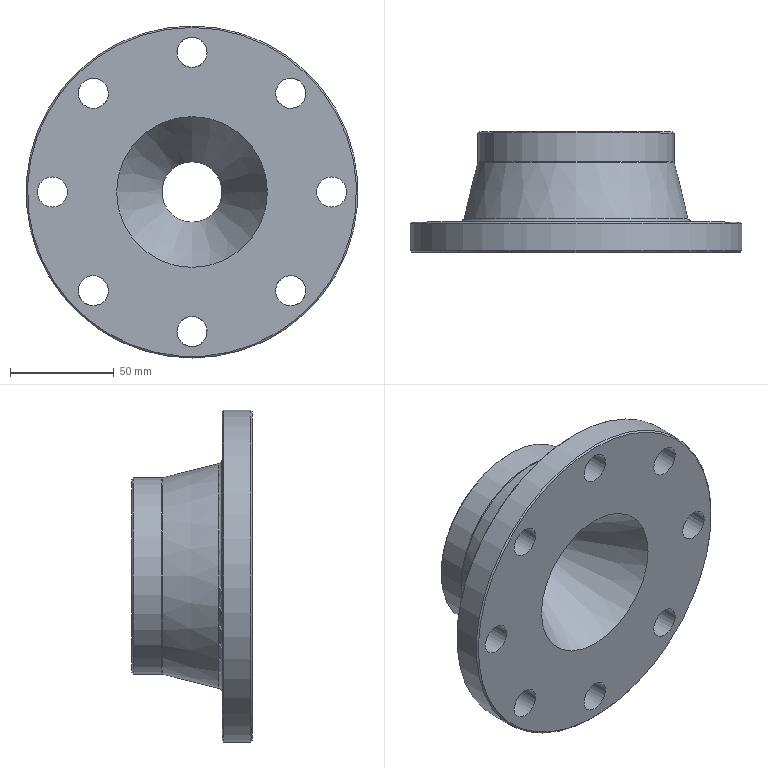Part | NX | features INSTANCE 8, ABSOLUTE_DATUM_PLANE 3, CHAMFER 2, DATUM_CSYS 2, SKETCH 2, ABSOLUTE_DATUM_AXIS 1, BLEND 1, CIRCULAR_ISET 1, HOLE PACKAGE 1, SCALE 1, SIMPLE HOLE 1, SWP104 1, TRANSFORM_ISET 1 | 1 solid | 21 faces | box 160 x 58.182 x 160 mm | volume 514948 mm3 | cylinder 11 | cone 5 | plane 3 | torus 2 | commonest cylinder face diameters 14.545 x8 29.091 x1 94.545 x1 160 x1
STEP:
#1=CARTESIAN_POINT('',(0.,17.422,79.273));
#2=VERTEX_POINT('',#1);
#3=CARTESIAN_POINT('',(0.,17.422,0.));
#4=DIRECTION('',(0.,1.,0.));
#5=DIRECTION('',(0.,0.,1.));
#6=AXIS2_PLACEMENT_3D('',#3,#4,#5);
#7=CIRCLE('',#6,79.273);
#8=EDGE_CURVE('',#2,#2,#7,.F.);
#9=ORIENTED_EDGE('',*,*,#8,.T.);
#10=EDGE_LOOP('',(#9));
#11=FACE_BOUND('',#10,.T.);
#12=CARTESIAN_POINT('',(47.569,17.422,54.842));
#13=VERTEX_POINT('',#12);
#14=CARTESIAN_POINT('',(47.569,17.422,47.569));
#15=DIRECTION('',(0.,1.,0.));
#16=DIRECTION('',(0.,0.,1.));
#17=AXIS2_PLACEMENT_3D('',#14,#15,#16);
#18=CIRCLE('',#17,7.273);
#19=EDGE_CURVE('',#13,#13,#18,.T.);
#20=ORIENTED_EDGE('',*,*,#19,.T.);
#21=EDGE_LOOP('',(#20));
#22=FACE_BOUND('',#21,.T.);
#23=CARTESIAN_POINT('',(0.,17.422,74.545));
#24=VERTEX_POINT('',#23);
#25=CARTESIAN_POINT('',(0.,17.422,67.273));
#26=DIRECTION('',(0.,1.,0.));
#27=DIRECTION('',(0.,0.,1.));
#28=AXIS2_PLACEMENT_3D('',#25,#26,#27);
#29=CIRCLE('',#28,7.273);
#30=EDGE_CURVE('',#24,#24,#29,.T.);
#31=ORIENTED_EDGE('',*,*,#30,.T.);
#32=EDGE_LOOP('',(#31));
#33=FACE_BOUND('',#32,.T.);
#34=CARTESIAN_POINT('',(-47.569,17.422,54.842));
#35=VERTEX_POINT('',#34);
#36=CARTESIAN_POINT('',(-47.569,17.422,47.569));
#37=DIRECTION('',(0.,1.,0.));
#38=DIRECTION('',(0.,0.,1.));
#39=AXIS2_PLACEMENT_3D('',#36,#37,#38);
#40=CIRCLE('',#39,7.273);
#41=EDGE_CURVE('',#35,#35,#40,.T.);
#42=ORIENTED_EDGE('',*,*,#41,.T.);
#43=EDGE_LOOP('',(#42));
#44=FACE_BOUND('',#43,.T.);
#45=CARTESIAN_POINT('',(-67.273,17.422,7.273));
#46=VERTEX_POINT('',#45);
#47=CARTESIAN_POINT('',(-67.273,17.422,0.));
#48=DIRECTION('',(0.,1.,0.));
#49=DIRECTION('',(0.,0.,1.));
#50=AXIS2_PLACEMENT_3D('',#47,#48,#49);
#51=CIRCLE('',#50,7.273);
#52=EDGE_CURVE('',#46,#46,#51,.T.);
#53=ORIENTED_EDGE('',*,*,#52,.T.);
#54=EDGE_LOOP('',(#53));
#55=FACE_BOUND('',#54,.T.);
#56=CARTESIAN_POINT('',(-47.569,17.422,-40.296));
#57=VERTEX_POINT('',#56);
#58=CARTESIAN_POINT('',(-47.569,17.422,-47.569));
#59=DIRECTION('',(0.,1.,0.));
#60=DIRECTION('',(0.,0.,1.));
#61=AXIS2_PLACEMENT_3D('',#58,#59,#60);
#62=CIRCLE('',#61,7.273);
#63=EDGE_CURVE('',#57,#57,#62,.T.);
#64=ORIENTED_EDGE('',*,*,#63,.T.);
#65=EDGE_LOOP('',(#64));
#66=FACE_BOUND('',#65,.T.);
#67=CARTESIAN_POINT('',(0.,17.422,-60.));
#68=VERTEX_POINT('',#67);
#69=CARTESIAN_POINT('',(0.,17.422,-67.273));
#70=DIRECTION('',(0.,1.,0.));
#71=DIRECTION('',(0.,0.,1.));
#72=AXIS2_PLACEMENT_3D('',#69,#70,#71);
#73=CIRCLE('',#72,7.273);
#74=EDGE_CURVE('',#68,#68,#73,.T.);
#75=ORIENTED_EDGE('',*,*,#74,.T.);
#76=EDGE_LOOP('',(#75));
#77=FACE_BOUND('',#76,.T.);
#78=CARTESIAN_POINT('',(47.569,17.422,-40.296));
#79=VERTEX_POINT('',#78);
#80=CARTESIAN_POINT('',(47.569,17.422,-47.569));
#81=DIRECTION('',(0.,1.,0.));
#82=DIRECTION('',(0.,0.,1.));
#83=AXIS2_PLACEMENT_3D('',#80,#81,#82);
#84=CIRCLE('',#83,7.273);
#85=EDGE_CURVE('',#79,#79,#84,.T.);
#86=ORIENTED_EDGE('',*,*,#85,.T.);
#87=EDGE_LOOP('',(#86));
#88=FACE_BOUND('',#87,.T.);
#89=CARTESIAN_POINT('',(67.273,17.422,7.273));
#90=VERTEX_POINT('',#89);
#91=CARTESIAN_POINT('',(67.273,17.422,0.));
#92=DIRECTION('',(0.,1.,0.));
#93=DIRECTION('',(0.,0.,1.));
#94=AXIS2_PLACEMENT_3D('',#91,#92,#93);
#95=CIRCLE('',#94,7.273);
#96=EDGE_CURVE('',#90,#90,#95,.T.);
#97=ORIENTED_EDGE('',*,*,#96,.T.);
#98=EDGE_LOOP('',(#97));
#99=FACE_BOUND('',#98,.T.);
#100=CARTESIAN_POINT('',(0.,17.422,-36.364));
#101=VERTEX_POINT('',#100);
#102=CARTESIAN_POINT('',(0.,17.422,0.));
#103=DIRECTION('',(0.,-1.,0.));
#104=DIRECTION('',(0.,0.,-1.));
#105=AXIS2_PLACEMENT_3D('',#102,#103,#104);
#106=CIRCLE('',#105,36.364);
#107=EDGE_CURVE('',#101,#101,#106,.T.);
#108=ORIENTED_EDGE('',*,*,#107,.F.);
#109=EDGE_LOOP('',(#108));
#110=FACE_BOUND('',#109,.T.);
#111=CARTESIAN_POINT('',(80.,17.422,0.));
#112=DIRECTION('',(0.,1.,0.));
#113=DIRECTION('',(0.,0.,1.));
#114=AXIS2_PLACEMENT_3D('',#111,#112,#113);
#115=PLANE('',#114);
#116=ADVANCED_FACE('',(#11,#22,#33,#44,#55,#66,#77,#88,#99,#110),#115,.F.);
#117=CARTESIAN_POINT('',(0.,56.695,-14.545));
#118=VERTEX_POINT('',#117);
#119=CARTESIAN_POINT('',(0.,56.695,0.));
#120=DIRECTION('',(0.,-1.,0.));
#121=DIRECTION('',(0.,0.,-1.));
#122=AXIS2_PLACEMENT_3D('',#119,#120,#121);
#123=CIRCLE('',#122,14.545);
#124=EDGE_CURVE('',#118,#118,#123,.T.);
#125=ORIENTED_EDGE('',*,*,#124,.F.);
#126=EDGE_LOOP('',(#125));
#127=FACE_BOUND('',#126,.T.);
#128=ORIENTED_EDGE('',*,*,#107,.T.);
#129=EDGE_LOOP('',(#128));
#130=FACE_BOUND('',#129,.T.);
#131=CARTESIAN_POINT('',(0.,17.422,0.));
#132=DIRECTION('',(0.,-1.,0.));
#133=DIRECTION('',(0.,0.,-1.));
#134=AXIS2_PLACEMENT_3D('',#131,#132,#133);
#135=CONICAL_SURFACE('',#134,36.364,0.5071);
#136=ADVANCED_FACE('',(#127,#130),#135,.F.);
#137=CARTESIAN_POINT('',(0.,75.604,-14.545));
#138=VERTEX_POINT('',#137);
#139=CARTESIAN_POINT('',(0.,75.604,0.));
#140=DIRECTION('',(0.,-1.,0.));
#141=DIRECTION('',(0.,0.,-1.));
#142=AXIS2_PLACEMENT_3D('',#139,#140,#141);
#143=CIRCLE('',#142,14.545);
#144=EDGE_CURVE('',#138,#138,#143,.T.);
#145=ORIENTED_EDGE('',*,*,#144,.F.);
#146=EDGE_LOOP('',(#145));
#147=FACE_BOUND('',#146,.T.);
#148=ORIENTED_EDGE('',*,*,#124,.T.);
#149=EDGE_LOOP('',(#148));
#150=FACE_BOUND('',#149,.T.);
#151=CARTESIAN_POINT('',(0.,0.,0.));
#152=DIRECTION('',(0.,-1.,0.));
#153=DIRECTION('',(0.,0.,-1.));
#154=AXIS2_PLACEMENT_3D('',#151,#152,#153);
#155=CYLINDRICAL_SURFACE('',#154,14.545);
#156=ADVANCED_FACE('',(#147,#150),#155,.F.);
#157=CARTESIAN_POINT('',(0.,75.604,-46.545));
#158=VERTEX_POINT('',#157);
#159=CARTESIAN_POINT('',(0.,75.604,0.));
#160=DIRECTION('',(0.,-1.,0.));
#161=DIRECTION('',(0.,0.,-1.));
#162=AXIS2_PLACEMENT_3D('',#159,#160,#161);
#163=CIRCLE('',#162,46.545);
#164=EDGE_CURVE('',#158,#158,#163,.F.);
#165=ORIENTED_EDGE('',*,*,#164,.T.);
#166=EDGE_LOOP('',(#165));
#167=FACE_BOUND('',#166,.T.);
#168=ORIENTED_EDGE('',*,*,#144,.T.);
#169=EDGE_LOOP('',(#168));
#170=FACE_BOUND('',#169,.T.);
#171=CARTESIAN_POINT('',(14.545,75.604,0.));
#172=DIRECTION('',(0.,-1.,0.));
#173=DIRECTION('',(0.,0.,-1.));
#174=AXIS2_PLACEMENT_3D('',#171,#172,#173);
#175=PLANE('',#174);
#176=ADVANCED_FACE('',(#167,#170),#175,.F.);
#177=CARTESIAN_POINT('',(0.,61.327,-47.273));
#178=VERTEX_POINT('',#177);
#179=CARTESIAN_POINT('',(0.,61.327,0.));
#180=DIRECTION('',(0.,-1.,0.));
#181=DIRECTION('',(0.,0.,-1.));
#182=AXIS2_PLACEMENT_3D('',#179,#180,#181);
#183=CIRCLE('',#182,47.273);
#184=EDGE_CURVE('',#178,#178,#183,.F.);
#185=ORIENTED_EDGE('',*,*,#184,.T.);
#186=EDGE_LOOP('',(#185));
#187=FACE_BOUND('',#186,.T.);
#188=CARTESIAN_POINT('',(0.,74.877,-47.273));
#189=VERTEX_POINT('',#188);
#190=CARTESIAN_POINT('',(0.,74.877,0.));
#191=DIRECTION('',(0.,-1.,0.));
#192=DIRECTION('',(0.,0.,-1.));
#193=AXIS2_PLACEMENT_3D('',#190,#191,#192);
#194=CIRCLE('',#193,47.273);
#195=EDGE_CURVE('',#189,#189,#194,.T.);
#196=ORIENTED_EDGE('',*,*,#195,.T.);
#197=EDGE_LOOP('',(#196));
#198=FACE_BOUND('',#197,.T.);
#199=CARTESIAN_POINT('',(0.,0.,0.));
#200=DIRECTION('',(0.,-1.,0.));
#201=DIRECTION('',(0.,0.,-1.));
#202=AXIS2_PLACEMENT_3D('',#199,#200,#201);
#203=CYLINDRICAL_SURFACE('',#202,47.273);
#204=ADVANCED_FACE('',(#187,#198),#203,.T.);
#205=CARTESIAN_POINT('',(0.,33.62,-54.132));
#206=VERTEX_POINT('',#205);
#207=CARTESIAN_POINT('',(0.,33.62,0.));
#208=DIRECTION('',(0.,-1.,0.));
#209=DIRECTION('',(0.,0.,-1.));
#210=AXIS2_PLACEMENT_3D('',#207,#208,#209);
#211=CIRCLE('',#210,54.132);
#212=EDGE_CURVE('',#206,#206,#211,.F.);
#213=ORIENTED_EDGE('',*,*,#212,.T.);
#214=EDGE_LOOP('',(#213));
#215=FACE_BOUND('',#214,.T.);
#216=CARTESIAN_POINT('',(0.,60.798,-47.338));
#217=VERTEX_POINT('',#216);
#218=CARTESIAN_POINT('',(0.,60.798,0.));
#219=DIRECTION('',(0.,-1.,0.));
#220=DIRECTION('',(0.,0.,-1.));
#221=AXIS2_PLACEMENT_3D('',#218,#219,#220);
#222=CIRCLE('',#221,47.338);
#223=EDGE_CURVE('',#217,#217,#222,.T.);
#224=ORIENTED_EDGE('',*,*,#223,.T.);
#225=EDGE_LOOP('',(#224));
#226=FACE_BOUND('',#225,.T.);
#227=CARTESIAN_POINT('',(0.,61.059,0.));
#228=DIRECTION('',(0.,-1.,0.));
#229=DIRECTION('',(0.,0.,-1.));
#230=AXIS2_PLACEMENT_3D('',#227,#228,#229);
#231=CONICAL_SURFACE('',#230,47.273,0.245);
#232=ADVANCED_FACE('',(#215,#226),#231,.T.);
#233=CARTESIAN_POINT('',(52.712,31.968,42.426));
#234=VERTEX_POINT('',#233);
#235=CARTESIAN_POINT('',(47.569,31.968,47.569));
#236=DIRECTION('',(0.,-1.,0.));
#237=DIRECTION('',(0.7071,0.,-0.7071));
#238=AXIS2_PLACEMENT_3D('',#235,#236,#237);
#239=CIRCLE('',#238,7.273);
#240=EDGE_CURVE('',#234,#234,#239,.T.);
#241=ORIENTED_EDGE('',*,*,#240,.T.);
#242=EDGE_LOOP('',(#241));
#243=FACE_BOUND('',#242,.T.);
#244=CARTESIAN_POINT('',(7.273,31.968,67.273));
#245=VERTEX_POINT('',#244);
#246=CARTESIAN_POINT('',(0.,31.968,67.273));
#247=DIRECTION('',(0.,-1.,0.));
#248=DIRECTION('',(1.,0.,0.));
#249=AXIS2_PLACEMENT_3D('',#246,#247,#248);
#250=CIRCLE('',#249,7.273);
#251=EDGE_CURVE('',#245,#245,#250,.T.);
#252=ORIENTED_EDGE('',*,*,#251,.T.);
#253=EDGE_LOOP('',(#252));
#254=FACE_BOUND('',#253,.T.);
#255=CARTESIAN_POINT('',(-42.426,31.968,52.712));
#256=VERTEX_POINT('',#255);
#257=CARTESIAN_POINT('',(-47.569,31.968,47.569));
#258=DIRECTION('',(0.,-1.,0.));
#259=DIRECTION('',(0.7071,0.,0.7071));
#260=AXIS2_PLACEMENT_3D('',#257,#258,#259);
#261=CIRCLE('',#260,7.273);
#262=EDGE_CURVE('',#256,#256,#261,.T.);
#263=ORIENTED_EDGE('',*,*,#262,.T.);
#264=EDGE_LOOP('',(#263));
#265=FACE_BOUND('',#264,.T.);
#266=CARTESIAN_POINT('',(-67.273,31.968,7.273));
#267=VERTEX_POINT('',#266);
#268=CARTESIAN_POINT('',(-67.273,31.968,0.));
#269=DIRECTION('',(0.,-1.,0.));
#270=DIRECTION('',(0.,0.,1.));
#271=AXIS2_PLACEMENT_3D('',#268,#269,#270);
#272=CIRCLE('',#271,7.273);
#273=EDGE_CURVE('',#267,#267,#272,.T.);
#274=ORIENTED_EDGE('',*,*,#273,.T.);
#275=EDGE_LOOP('',(#274));
#276=FACE_BOUND('',#275,.T.);
#277=CARTESIAN_POINT('',(-52.712,31.968,-42.426));
#278=VERTEX_POINT('',#277);
#279=CARTESIAN_POINT('',(-47.569,31.968,-47.569));
#280=DIRECTION('',(0.,-1.,0.));
#281=DIRECTION('',(-0.7071,0.,0.7071));
#282=AXIS2_PLACEMENT_3D('',#279,#280,#281);
#283=CIRCLE('',#282,7.273);
#284=EDGE_CURVE('',#278,#278,#283,.T.);
#285=ORIENTED_EDGE('',*,*,#284,.T.);
#286=EDGE_LOOP('',(#285));
#287=FACE_BOUND('',#286,.T.);
#288=CARTESIAN_POINT('',(-7.273,31.968,-67.273));
#289=VERTEX_POINT('',#288);
#290=CARTESIAN_POINT('',(0.,31.968,-67.273));
#291=DIRECTION('',(0.,-1.,0.));
#292=DIRECTION('',(-1.,0.,0.));
#293=AXIS2_PLACEMENT_3D('',#290,#291,#292);
#294=CIRCLE('',#293,7.273);
#295=EDGE_CURVE('',#289,#289,#294,.T.);
#296=ORIENTED_EDGE('',*,*,#295,.T.);
#297=EDGE_LOOP('',(#296));
#298=FACE_BOUND('',#297,.T.);
#299=CARTESIAN_POINT('',(42.426,31.968,-52.712));
#300=VERTEX_POINT('',#299);
#301=CARTESIAN_POINT('',(47.569,31.968,-47.569));
#302=DIRECTION('',(0.,-1.,0.));
#303=DIRECTION('',(-0.7071,0.,-0.7071));
#304=AXIS2_PLACEMENT_3D('',#301,#302,#303);
#305=CIRCLE('',#304,7.273);
#306=EDGE_CURVE('',#300,#300,#305,.T.);
#307=ORIENTED_EDGE('',*,*,#306,.T.);
#308=EDGE_LOOP('',(#307));
#309=FACE_BOUND('',#308,.T.);
#310=CARTESIAN_POINT('',(67.273,31.968,-7.273));
#311=VERTEX_POINT('',#310);
#312=CARTESIAN_POINT('',(67.273,31.968,0.));
#313=DIRECTION('',(0.,-1.,0.));
#314=DIRECTION('',(0.,0.,-1.));
#315=AXIS2_PLACEMENT_3D('',#312,#313,#314);
#316=CIRCLE('',#315,7.273);
#317=EDGE_CURVE('',#311,#311,#316,.T.);
#318=ORIENTED_EDGE('',*,*,#317,.T.);
#319=EDGE_LOOP('',(#318));
#320=FACE_BOUND('',#319,.T.);
#321=CARTESIAN_POINT('',(0.,31.968,-56.249));
#322=VERTEX_POINT('',#321);
#323=CARTESIAN_POINT('',(0.,31.968,0.));
#324=DIRECTION('',(0.,-1.,0.));
#325=DIRECTION('',(0.,0.,-1.));
#326=AXIS2_PLACEMENT_3D('',#323,#324,#325);
#327=CIRCLE('',#326,56.249);
#328=EDGE_CURVE('',#322,#322,#327,.T.);
#329=ORIENTED_EDGE('',*,*,#328,.T.);
#330=EDGE_LOOP('',(#329));
#331=FACE_BOUND('',#330,.T.);
#332=CARTESIAN_POINT('',(0.,31.968,-79.273));
#333=VERTEX_POINT('',#332);
#334=CARTESIAN_POINT('',(0.,31.968,0.));
#335=DIRECTION('',(0.,-1.,0.));
#336=DIRECTION('',(0.,0.,-1.));
#337=AXIS2_PLACEMENT_3D('',#334,#335,#336);
#338=CIRCLE('',#337,79.273);
#339=EDGE_CURVE('',#333,#333,#338,.F.);
#340=ORIENTED_EDGE('',*,*,#339,.T.);
#341=EDGE_LOOP('',(#340));
#342=FACE_BOUND('',#341,.T.);
#343=CARTESIAN_POINT('',(54.545,31.968,0.));
#344=DIRECTION('',(0.,-1.,0.));
#345=DIRECTION('',(0.,0.,-1.));
#346=AXIS2_PLACEMENT_3D('',#343,#344,#345);
#347=PLANE('',#346);
#348=ADVANCED_FACE('',(#243,#254,#265,#276,#287,#298,#309,#320,#331,#342),#347,.F.);
#349=CARTESIAN_POINT('',(0.,18.15,80.));
#350=VERTEX_POINT('',#349);
#351=CARTESIAN_POINT('',(0.,18.15,0.));
#352=DIRECTION('',(0.,1.,0.));
#353=DIRECTION('',(0.,0.,1.));
#354=AXIS2_PLACEMENT_3D('',#351,#352,#353);
#355=CIRCLE('',#354,80.);
#356=EDGE_CURVE('',#350,#350,#355,.T.);
#357=ORIENTED_EDGE('',*,*,#356,.T.);
#358=EDGE_LOOP('',(#357));
#359=FACE_BOUND('',#358,.T.);
#360=CARTESIAN_POINT('',(0.,31.24,-80.));
#361=VERTEX_POINT('',#360);
#362=CARTESIAN_POINT('',(0.,31.24,0.));
#363=DIRECTION('',(0.,-1.,0.));
#364=DIRECTION('',(0.,0.,-1.));
#365=AXIS2_PLACEMENT_3D('',#362,#363,#364);
#366=CIRCLE('',#365,80.);
#367=EDGE_CURVE('',#361,#361,#366,.T.);
#368=ORIENTED_EDGE('',*,*,#367,.T.);
#369=EDGE_LOOP('',(#368));
#370=FACE_BOUND('',#369,.T.);
#371=CARTESIAN_POINT('',(0.,0.,0.));
#372=DIRECTION('',(0.,-1.,0.));
#373=DIRECTION('',(0.,0.,-1.));
#374=AXIS2_PLACEMENT_3D('',#371,#372,#373);
#375=CYLINDRICAL_SURFACE('',#374,80.);
#376=ADVANCED_FACE('',(#359,#370),#375,.T.);
#377=ORIENTED_EDGE('',*,*,#164,.F.);
#378=EDGE_LOOP('',(#377));
#379=FACE_BOUND('',#378,.T.);
#380=ORIENTED_EDGE('',*,*,#195,.F.);
#381=EDGE_LOOP('',(#380));
#382=FACE_BOUND('',#381,.T.);
#383=CARTESIAN_POINT('',(0.,74.877,0.));
#384=DIRECTION('',(0.,-1.,0.));
#385=DIRECTION('',(0.,0.,-1.));
#386=AXIS2_PLACEMENT_3D('',#383,#384,#385);
#387=CONICAL_SURFACE('',#386,47.273,0.7854);
#388=ADVANCED_FACE('',(#379,#382),#387,.T.);
#389=ORIENTED_EDGE('',*,*,#339,.F.);
#390=EDGE_LOOP('',(#389));
#391=FACE_BOUND('',#390,.T.);
#392=ORIENTED_EDGE('',*,*,#367,.F.);
#393=EDGE_LOOP('',(#392));
#394=FACE_BOUND('',#393,.T.);
#395=CARTESIAN_POINT('',(0.,31.24,0.));
#396=DIRECTION('',(0.,-1.,0.));
#397=DIRECTION('',(0.,0.,-1.));
#398=AXIS2_PLACEMENT_3D('',#395,#396,#397);
#399=CONICAL_SURFACE('',#398,80.,0.7854);
#400=ADVANCED_FACE('',(#391,#394),#399,.T.);
#401=ORIENTED_EDGE('',*,*,#212,.F.);
#402=EDGE_LOOP('',(#401));
#403=FACE_BOUND('',#402,.T.);
#404=ORIENTED_EDGE('',*,*,#328,.F.);
#405=EDGE_LOOP('',(#404));
#406=FACE_BOUND('',#405,.T.);
#407=CARTESIAN_POINT('',(0.,34.15,0.));
#408=DIRECTION('',(0.,-1.,0.));
#409=DIRECTION('',(0.,0.,-1.));
#410=AXIS2_PLACEMENT_3D('',#407,#408,#409);
#411=TOROIDAL_SURFACE('',#410,56.249,2.182);
#412=ADVANCED_FACE('',(#403,#406),#411,.F.);
#413=ORIENTED_EDGE('',*,*,#184,.F.);
#414=EDGE_LOOP('',(#413));
#415=FACE_BOUND('',#414,.T.);
#416=ORIENTED_EDGE('',*,*,#223,.F.);
#417=EDGE_LOOP('',(#416));
#418=FACE_BOUND('',#417,.T.);
#419=CARTESIAN_POINT('',(0.,61.327,0.));
#420=DIRECTION('',(0.,-1.,0.));
#421=DIRECTION('',(0.,0.,-1.));
#422=AXIS2_PLACEMENT_3D('',#419,#420,#421);
#423=TOROIDAL_SURFACE('',#422,49.455,2.182);
#424=ADVANCED_FACE('',(#415,#418),#423,.F.);
#425=ORIENTED_EDGE('',*,*,#317,.F.);
#426=EDGE_LOOP('',(#425));
#427=FACE_BOUND('',#426,.T.);
#428=ORIENTED_EDGE('',*,*,#96,.F.);
#429=EDGE_LOOP('',(#428));
#430=FACE_BOUND('',#429,.T.);
#431=CARTESIAN_POINT('',(67.273,31.968,0.));
#432=DIRECTION('',(0.,-1.,0.));
#433=DIRECTION('',(0.,0.,-1.));
#434=AXIS2_PLACEMENT_3D('',#431,#432,#433);
#435=CYLINDRICAL_SURFACE('',#434,7.273);
#436=ADVANCED_FACE('',(#427,#430),#435,.F.);
#437=ORIENTED_EDGE('',*,*,#306,.F.);
#438=EDGE_LOOP('',(#437));
#439=FACE_BOUND('',#438,.T.);
#440=ORIENTED_EDGE('',*,*,#85,.F.);
#441=EDGE_LOOP('',(#440));
#442=FACE_BOUND('',#441,.T.);
#443=CARTESIAN_POINT('',(47.569,31.968,-47.569));
#444=DIRECTION('',(0.,-1.,0.));
#445=DIRECTION('',(-0.7071,0.,-0.7071));
#446=AXIS2_PLACEMENT_3D('',#443,#444,#445);
#447=CYLINDRICAL_SURFACE('',#446,7.273);
#448=ADVANCED_FACE('',(#439,#442),#447,.F.);
#449=ORIENTED_EDGE('',*,*,#295,.F.);
#450=EDGE_LOOP('',(#449));
#451=FACE_BOUND('',#450,.T.);
#452=ORIENTED_EDGE('',*,*,#74,.F.);
#453=EDGE_LOOP('',(#452));
#454=FACE_BOUND('',#453,.T.);
#455=CARTESIAN_POINT('',(0.,31.968,-67.273));
#456=DIRECTION('',(0.,-1.,0.));
#457=DIRECTION('',(-1.,0.,0.));
#458=AXIS2_PLACEMENT_3D('',#455,#456,#457);
#459=CYLINDRICAL_SURFACE('',#458,7.273);
#460=ADVANCED_FACE('',(#451,#454),#459,.F.);
#461=ORIENTED_EDGE('',*,*,#284,.F.);
#462=EDGE_LOOP('',(#461));
#463=FACE_BOUND('',#462,.T.);
#464=ORIENTED_EDGE('',*,*,#63,.F.);
#465=EDGE_LOOP('',(#464));
#466=FACE_BOUND('',#465,.T.);
#467=CARTESIAN_POINT('',(-47.569,31.968,-47.569));
#468=DIRECTION('',(0.,-1.,0.));
#469=DIRECTION('',(-0.7071,0.,0.7071));
#470=AXIS2_PLACEMENT_3D('',#467,#468,#469);
#471=CYLINDRICAL_SURFACE('',#470,7.273);
#472=ADVANCED_FACE('',(#463,#466),#471,.F.);
#473=ORIENTED_EDGE('',*,*,#273,.F.);
#474=EDGE_LOOP('',(#473));
#475=FACE_BOUND('',#474,.T.);
#476=ORIENTED_EDGE('',*,*,#52,.F.);
#477=EDGE_LOOP('',(#476));
#478=FACE_BOUND('',#477,.T.);
#479=CARTESIAN_POINT('',(-67.273,31.968,0.));
#480=DIRECTION('',(0.,-1.,0.));
#481=DIRECTION('',(0.,0.,1.));
#482=AXIS2_PLACEMENT_3D('',#479,#480,#481);
#483=CYLINDRICAL_SURFACE('',#482,7.273);
#484=ADVANCED_FACE('',(#475,#478),#483,.F.);
#485=ORIENTED_EDGE('',*,*,#262,.F.);
#486=EDGE_LOOP('',(#485));
#487=FACE_BOUND('',#486,.T.);
#488=ORIENTED_EDGE('',*,*,#41,.F.);
#489=EDGE_LOOP('',(#488));
#490=FACE_BOUND('',#489,.T.);
#491=CARTESIAN_POINT('',(-47.569,31.968,47.569));
#492=DIRECTION('',(0.,-1.,0.));
#493=DIRECTION('',(0.7071,0.,0.7071));
#494=AXIS2_PLACEMENT_3D('',#491,#492,#493);
#495=CYLINDRICAL_SURFACE('',#494,7.273);
#496=ADVANCED_FACE('',(#487,#490),#495,.F.);
#497=ORIENTED_EDGE('',*,*,#251,.F.);
#498=EDGE_LOOP('',(#497));
#499=FACE_BOUND('',#498,.T.);
#500=ORIENTED_EDGE('',*,*,#30,.F.);
#501=EDGE_LOOP('',(#500));
#502=FACE_BOUND('',#501,.T.);
#503=CARTESIAN_POINT('',(0.,31.968,67.273));
#504=DIRECTION('',(0.,-1.,0.));
#505=DIRECTION('',(1.,0.,0.));
#506=AXIS2_PLACEMENT_3D('',#503,#504,#505);
#507=CYLINDRICAL_SURFACE('',#506,7.273);
#508=ADVANCED_FACE('',(#499,#502),#507,.F.);
#509=ORIENTED_EDGE('',*,*,#240,.F.);
#510=EDGE_LOOP('',(#509));
#511=FACE_BOUND('',#510,.T.);
#512=ORIENTED_EDGE('',*,*,#19,.F.);
#513=EDGE_LOOP('',(#512));
#514=FACE_BOUND('',#513,.T.);
#515=CARTESIAN_POINT('',(47.569,31.968,47.569));
#516=DIRECTION('',(0.,-1.,0.));
#517=DIRECTION('',(0.7071,0.,-0.7071));
#518=AXIS2_PLACEMENT_3D('',#515,#516,#517);
#519=CYLINDRICAL_SURFACE('',#518,7.273);
#520=ADVANCED_FACE('',(#511,#514),#519,.F.);
#521=ORIENTED_EDGE('',*,*,#356,.F.);
#522=EDGE_LOOP('',(#521));
#523=FACE_BOUND('',#522,.T.);
#524=ORIENTED_EDGE('',*,*,#8,.F.);
#525=EDGE_LOOP('',(#524));
#526=FACE_BOUND('',#525,.T.);
#527=CARTESIAN_POINT('',(0.,17.422,0.));
#528=DIRECTION('',(0.,1.,0.));
#529=DIRECTION('',(0.,0.,1.));
#530=AXIS2_PLACEMENT_3D('',#527,#528,#529);
#531=CONICAL_SURFACE('',#530,79.273,0.7854);
#532=ADVANCED_FACE('',(#523,#526),#531,.T.);
#533=CLOSED_SHELL('',(#116,#136,#156,#176,#204,#232,#348,#376,#388,#400,#412,#424,#436,#448,#460,#472,#484,#496,#508,#520,#532));
#534=MANIFOLD_SOLID_BREP('',#533);
#535=(LENGTH_UNIT()NAMED_UNIT(*)SI_UNIT(.MILLI.,.METRE.));
#536=UNCERTAINTY_MEASURE_WITH_UNIT(LENGTH_MEASURE(0.00001),#535,'','');
#537=(NAMED_UNIT(*)PLANE_ANGLE_UNIT()SI_UNIT($,.RADIAN.));
#538=(NAMED_UNIT(*)SI_UNIT($,.STERADIAN.)SOLID_ANGLE_UNIT());
#539=(GEOMETRIC_REPRESENTATION_CONTEXT(3)GLOBAL_UNCERTAINTY_ASSIGNED_CONTEXT((#536))GLOBAL_UNIT_ASSIGNED_CONTEXT((#535,#537,#538))REPRESENTATION_CONTEXT('',''));
#540=ADVANCED_BREP_SHAPE_REPRESENTATION('',(#534),#539);